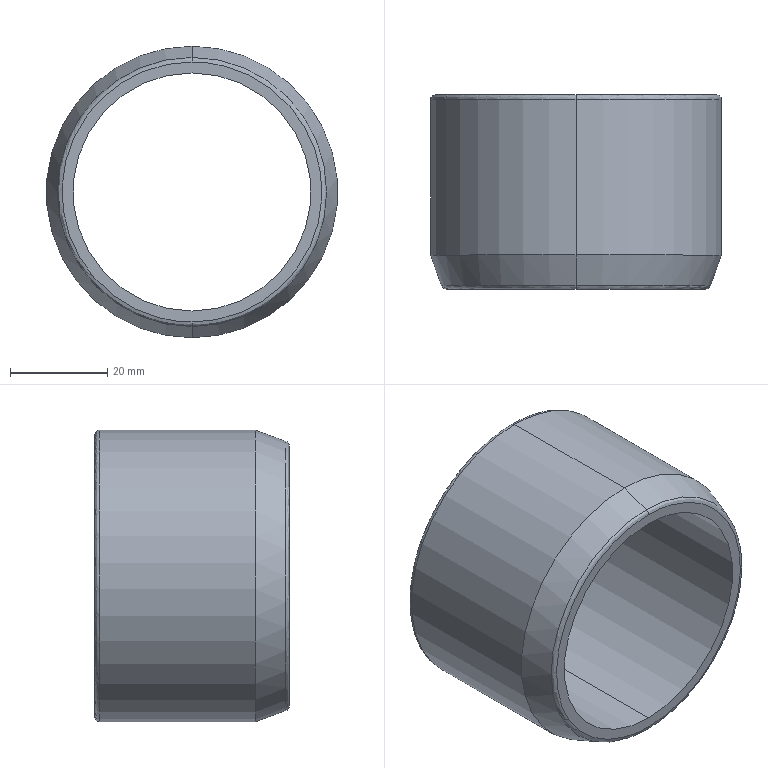Part | STEP file | 4. Piston Cap | 1 solid | 12 faces | box 60 x 40 x 60 mm | volume 35974 mm3 | spline 4 | cylinder 4 | cone 2 | plane 2 | commonest cylinder face diameters 49 x2 60 x2
STEP:
#1=CARTESIAN_POINT('',(0.,0.,26.752));
#2=VERTEX_POINT('',#1);
#3=CARTESIAN_POINT('',(0.,0.,-26.752));
#4=VERTEX_POINT('',#3);
#5=CARTESIAN_POINT('',(0.,0.,26.752));
#6=CARTESIAN_POINT('',(-0.818,0.,26.752));
#7=CARTESIAN_POINT('',(-2.04,0.,26.696));
#8=CARTESIAN_POINT('',(-3.457,0.,26.533));
#9=CARTESIAN_POINT('',(-4.163,0.,26.428));
#10=CARTESIAN_POINT('',(-4.516,0.,26.368));
#11=CARTESIAN_POINT('',(-4.692,0.,26.337));
#12=CARTESIAN_POINT('',(-4.767,0.,26.324));
#13=CARTESIAN_POINT('',(-4.818,0.,26.315));
#14=CARTESIAN_POINT('',(-4.841,0.,26.31));
#15=CARTESIAN_POINT('',(-5.721,0.,26.148));
#16=CARTESIAN_POINT('',(-6.983,0.,25.85));
#17=CARTESIAN_POINT('',(-8.425,0.,25.397));
#18=CARTESIAN_POINT('',(-9.139,0.,25.144));
#19=CARTESIAN_POINT('',(-9.494,0.,25.011));
#20=CARTESIAN_POINT('',(-9.671,0.,24.943));
#21=CARTESIAN_POINT('',(-9.746,0.,24.913));
#22=CARTESIAN_POINT('',(-9.797,0.,24.894));
#23=CARTESIAN_POINT('',(-9.821,0.,24.884));
#24=CARTESIAN_POINT('',(-10.688,0.,24.541));
#25=CARTESIAN_POINT('',(-11.917,0.,23.981));
#26=CARTESIAN_POINT('',(-13.296,0.,23.222));
#27=CARTESIAN_POINT('',(-13.972,0.,22.815));
#28=CARTESIAN_POINT('',(-14.307,0.,22.606));
#29=CARTESIAN_POINT('',(-14.449,0.,22.514));
#30=CARTESIAN_POINT('',(-14.544,0.,22.453));
#31=CARTESIAN_POINT('',(-14.591,0.,22.423));
#32=CARTESIAN_POINT('',(-16.184,0.,21.381));
#33=CARTESIAN_POINT('',(-17.611,0.,20.222));
#34=CARTESIAN_POINT('',(-19.569,0.,18.264));
#35=CARTESIAN_POINT('',(-20.493,0.,17.239));
#36=CARTESIAN_POINT('',(-21.475,0.,15.965));
#37=CARTESIAN_POINT('',(-21.941,0.,15.309));
#38=CARTESIAN_POINT('',(-22.168,0.,14.976));
#39=CARTESIAN_POINT('',(-22.264,0.,14.832));
#40=CARTESIAN_POINT('',(-22.328,0.,14.735));
#41=CARTESIAN_POINT('',(-22.36,0.,14.686));
#42=CARTESIAN_POINT('',(-22.886,0.,13.882));
#43=CARTESIAN_POINT('',(-23.567,0.,12.716));
#44=CARTESIAN_POINT('',(-24.256,0.,11.3));
#45=CARTESIAN_POINT('',(-24.574,0.,10.578));
#46=CARTESIAN_POINT('',(-24.726,0.,10.214));
#47=CARTESIAN_POINT('',(-24.8,0.,10.031));
#48=CARTESIAN_POINT('',(-24.832,0.,9.952));
#49=CARTESIAN_POINT('',(-24.853,0.,9.9));
#50=CARTESIAN_POINT('',(-24.864,0.,9.872));
#51=CARTESIAN_POINT('',(-25.193,0.,9.041));
#52=CARTESIAN_POINT('',(-25.611,0.,7.813));
#53=CARTESIAN_POINT('',(-25.994,0.,6.351));
#54=CARTESIAN_POINT('',(-26.158,0.,5.612));
#55=CARTESIAN_POINT('',(-26.234,0.,5.241));
#56=CARTESIAN_POINT('',(-26.27,0.,5.054));
#57=CARTESIAN_POINT('',(-26.285,0.,4.974));
#58=CARTESIAN_POINT('',(-26.295,0.,4.921));
#59=CARTESIAN_POINT('',(-26.301,0.,4.893));
#60=CARTESIAN_POINT('',(-26.603,0.,3.259));
#61=CARTESIAN_POINT('',(-26.752,0.,1.636));
#62=CARTESIAN_POINT('',(-26.752,0.,-0.818));
#63=CARTESIAN_POINT('',(-26.696,0.,-2.04));
#64=CARTESIAN_POINT('',(-26.533,0.,-3.457));
#65=CARTESIAN_POINT('',(-26.428,0.,-4.163));
#66=CARTESIAN_POINT('',(-26.368,0.,-4.516));
#67=CARTESIAN_POINT('',(-26.337,0.,-4.692));
#68=CARTESIAN_POINT('',(-26.324,0.,-4.767));
#69=CARTESIAN_POINT('',(-26.315,0.,-4.818));
#70=CARTESIAN_POINT('',(-26.31,0.,-4.841));
#71=CARTESIAN_POINT('',(-26.148,0.,-5.721));
#72=CARTESIAN_POINT('',(-25.85,0.,-6.983));
#73=CARTESIAN_POINT('',(-25.397,0.,-8.425));
#74=CARTESIAN_POINT('',(-25.144,0.,-9.139));
#75=CARTESIAN_POINT('',(-25.011,0.,-9.494));
#76=CARTESIAN_POINT('',(-24.943,0.,-9.671));
#77=CARTESIAN_POINT('',(-24.913,0.,-9.746));
#78=CARTESIAN_POINT('',(-24.894,0.,-9.797));
#79=CARTESIAN_POINT('',(-24.884,0.,-9.821));
#80=CARTESIAN_POINT('',(-24.541,0.,-10.688));
#81=CARTESIAN_POINT('',(-23.981,0.,-11.917));
#82=CARTESIAN_POINT('',(-23.222,0.,-13.296));
#83=CARTESIAN_POINT('',(-22.815,0.,-13.972));
#84=CARTESIAN_POINT('',(-22.606,0.,-14.307));
#85=CARTESIAN_POINT('',(-22.514,0.,-14.449));
#86=CARTESIAN_POINT('',(-22.453,0.,-14.544));
#87=CARTESIAN_POINT('',(-22.423,0.,-14.591));
#88=CARTESIAN_POINT('',(-21.381,0.,-16.184));
#89=CARTESIAN_POINT('',(-20.222,0.,-17.611));
#90=CARTESIAN_POINT('',(-18.264,0.,-19.569));
#91=CARTESIAN_POINT('',(-17.239,0.,-20.493));
#92=CARTESIAN_POINT('',(-15.965,0.,-21.475));
#93=CARTESIAN_POINT('',(-15.309,0.,-21.941));
#94=CARTESIAN_POINT('',(-14.976,0.,-22.168));
#95=CARTESIAN_POINT('',(-14.832,0.,-22.264));
#96=CARTESIAN_POINT('',(-14.735,0.,-22.328));
#97=CARTESIAN_POINT('',(-14.686,0.,-22.36));
#98=CARTESIAN_POINT('',(-13.882,0.,-22.886));
#99=CARTESIAN_POINT('',(-12.716,0.,-23.567));
#100=CARTESIAN_POINT('',(-11.3,0.,-24.256));
#101=CARTESIAN_POINT('',(-10.578,0.,-24.574));
#102=CARTESIAN_POINT('',(-10.214,0.,-24.726));
#103=CARTESIAN_POINT('',(-10.031,0.,-24.8));
#104=CARTESIAN_POINT('',(-9.952,0.,-24.832));
#105=CARTESIAN_POINT('',(-9.9,0.,-24.853));
#106=CARTESIAN_POINT('',(-9.872,0.,-24.864));
#107=CARTESIAN_POINT('',(-9.041,0.,-25.193));
#108=CARTESIAN_POINT('',(-7.813,0.,-25.611));
#109=CARTESIAN_POINT('',(-6.351,0.,-25.994));
#110=CARTESIAN_POINT('',(-5.612,0.,-26.158));
#111=CARTESIAN_POINT('',(-5.241,0.,-26.234));
#112=CARTESIAN_POINT('',(-5.054,0.,-26.27));
#113=CARTESIAN_POINT('',(-4.974,0.,-26.285));
#114=CARTESIAN_POINT('',(-4.921,0.,-26.295));
#115=CARTESIAN_POINT('',(-4.893,0.,-26.301));
#116=CARTESIAN_POINT('',(-3.259,0.,-26.603));
#117=CARTESIAN_POINT('',(-1.636,0.,-26.752));
#118=CARTESIAN_POINT('',(0.,0.,-26.752));
#119=B_SPLINE_CURVE_WITH_KNOTS('',3,(#5,#6,#7,#8,#9,#10,#11,#12,#13,#14,#15,#16,#17,#18,#19,#20,#21,#22,#23,#24,#25,#26,#27,#28,#29,#30,#31,#32,#33,#34,#35,#36,#37,#38,#39,#40,#41,#42,#43,#44,#45,#46,#47,#48,#49,#50,#51,#52,#53,#54,#55,#56,#57,#58,#59,#60,#61,#62,#63,#64,#65,#66,#67,#68,#69,#70,#71,#72,#73,#74,#75,#76,#77,#78,#79,#80,#81,#82,#83,#84,#85,#86,#87,#88,#89,#90,#91,#92,#93,#94,#95,#96,#97,#98,#99,#100,#101,#102,#103,#104,#105,#106,#107,#108,#109,#110,#111,#112,#113,#114,#115,#116,#117,#118),.UNSPECIFIED.,.F.,.F.,(4,1,1,1,1,1,2,2,1,1,1,1,1,2,2,1,1,1,1,2,2,2,1,1,1,1,2,2,1,1,1,1,1,2,2,1,1,1,1,1,2,2,2,1,1,1,1,1,2,2,1,1,1,1,1,2,2,1,1,1,1,2,2,2,1,1,1,1,2,2,1,1,1,1,1,2,2,1,1,1,1,1,2,2,4),(0.5,0.5156,0.5234,0.5273,0.5293,0.5303,0.5308,0.5312,0.5469,0.5547,0.5586,0.5605,0.5615,0.562,0.5625,0.5781,0.5859,0.5898,0.5918,0.5928,0.5938,0.625,0.6406,0.6484,0.6523,0.6543,0.6553,0.6563,0.6719,0.6797,0.6836,0.6855,0.6865,0.687,0.6875,0.7031,0.7109,0.7148,0.7168,0.7178,0.7183,0.7188,0.75,0.7656,0.7734,0.7773,0.7793,0.7803,0.7808,0.7813,0.7969,0.8047,0.8086,0.8105,0.8115,0.812,0.8125,0.8281,0.8359,0.8398,0.8418,0.8428,0.8438,0.875,0.8906,0.8984,0.9023,0.9043,0.9053,0.9063,0.9219,0.9297,0.9336,0.9355,0.9365,0.937,0.9375,0.9531,0.9609,0.9648,0.9668,0.9678,0.9683,0.9687,1.),.UNSPECIFIED.);
#120=EDGE_CURVE('',#2,#4,#119,.T.);
#121=ORIENTED_EDGE('',*,*,#120,.F.);
#122=CARTESIAN_POINT('',(0.,0.658,27.692));
#123=VERTEX_POINT('',#122);
#124=CARTESIAN_POINT('',(0.,1.,26.752));
#125=DIRECTION('',(-1.,0.,0.));
#126=DIRECTION('',(0.,0.,1.));
#127=AXIS2_PLACEMENT_3D('',#124,#125,#126);
#128=CIRCLE('',#127,1.);
#129=EDGE_CURVE('',#2,#123,#128,.T.);
#130=ORIENTED_EDGE('',*,*,#129,.T.);
#131=CARTESIAN_POINT('',(0.,0.658,-27.692));
#132=VERTEX_POINT('',#131);
#133=CARTESIAN_POINT('',(0.,0.658,0.));
#134=DIRECTION('',(0.,-1.,0.));
#135=DIRECTION('',(0.,0.,-1.));
#136=AXIS2_PLACEMENT_3D('',#133,#134,#135);
#137=CIRCLE('',#136,27.692);
#138=EDGE_CURVE('',#123,#132,#137,.T.);
#139=ORIENTED_EDGE('',*,*,#138,.T.);
#140=CARTESIAN_POINT('',(0.,1.,-26.752));
#141=DIRECTION('',(1.,0.,0.));
#142=DIRECTION('',(0.,0.,-1.));
#143=AXIS2_PLACEMENT_3D('',#140,#141,#142);
#144=CIRCLE('',#143,1.);
#145=EDGE_CURVE('',#4,#132,#144,.T.);
#146=ORIENTED_EDGE('',*,*,#145,.F.);
#147=EDGE_LOOP('',(#121,#130,#139,#146));
#148=FACE_OUTER_BOUND('',#147,.T.);
#149=CARTESIAN_POINT('',(0.,0.,26.752));
#150=CARTESIAN_POINT('',(-53.504,0.,26.752));
#151=CARTESIAN_POINT('',(-53.504,0.,-26.752));
#152=CARTESIAN_POINT('',(0.,0.,-26.752));
#153=CARTESIAN_POINT('',(0.,0.,27.187));
#154=CARTESIAN_POINT('',(-54.374,0.,27.187));
#155=CARTESIAN_POINT('',(-54.374,0.,-27.187));
#156=CARTESIAN_POINT('',(0.,0.,-27.187));
#157=CARTESIAN_POINT('',(0.,0.2494,27.543));
#158=CARTESIAN_POINT('',(-55.086,0.2494,27.543));
#159=CARTESIAN_POINT('',(-55.086,0.2494,-27.543));
#160=CARTESIAN_POINT('',(0.,0.2494,-27.543));
#161=CARTESIAN_POINT('',(0.,0.658,27.692));
#162=CARTESIAN_POINT('',(-55.383,0.658,27.692));
#163=CARTESIAN_POINT('',(-55.383,0.658,-27.692));
#164=CARTESIAN_POINT('',(0.,0.658,-27.692));
#165=(BOUNDED_SURFACE()B_SPLINE_SURFACE(3,3,((#149,#150,#151,#152),(#153,#154,#155,#156),(#157,#158,#159,#160),(#161,#162,#163,#164)),.UNSPECIFIED.,.F.,.F.,.F.)B_SPLINE_SURFACE_WITH_KNOTS((4,4),(4,4),(0.,1.),(0.,1.),.UNSPECIFIED.)GEOMETRIC_REPRESENTATION_ITEM()RATIONAL_B_SPLINE_SURFACE(((1.,0.3333,0.3333,1.),(0.8794,0.2931,0.2931,0.8794),(0.8794,0.2931,0.2931,0.8794),(1.,0.3333,0.3333,1.)))REPRESENTATION_ITEM('')SURFACE());
#166=ADVANCED_FACE('',(#148),#165,.T.);
#167=CARTESIAN_POINT('',(0.,39.,-30.));
#168=VERTEX_POINT('',#167);
#169=CARTESIAN_POINT('',(0.,39.,30.));
#170=VERTEX_POINT('',#169);
#171=CARTESIAN_POINT('',(0.,39.,0.));
#172=DIRECTION('',(0.,1.,0.));
#173=DIRECTION('',(0.,0.,-1.));
#174=AXIS2_PLACEMENT_3D('',#171,#172,#173);
#175=CIRCLE('',#174,30.);
#176=EDGE_CURVE('',#168,#170,#175,.T.);
#177=ORIENTED_EDGE('',*,*,#176,.T.);
#178=CARTESIAN_POINT('',(0.,40.,29.));
#179=VERTEX_POINT('',#178);
#180=CARTESIAN_POINT('',(0.,39.,29.));
#181=DIRECTION('',(-1.,0.,0.));
#182=DIRECTION('',(0.,0.,1.));
#183=AXIS2_PLACEMENT_3D('',#180,#181,#182);
#184=CIRCLE('',#183,1.);
#185=EDGE_CURVE('',#170,#179,#184,.T.);
#186=ORIENTED_EDGE('',*,*,#185,.T.);
#187=CARTESIAN_POINT('',(0.,40.,-29.));
#188=VERTEX_POINT('',#187);
#189=CARTESIAN_POINT('',(0.,40.,29.));
#190=CARTESIAN_POINT('',(-58.,40.,29.));
#191=CARTESIAN_POINT('',(-58.,40.,-29.));
#192=CARTESIAN_POINT('',(0.,40.,-29.));
#193=(BOUNDED_CURVE()B_SPLINE_CURVE(3,(#189,#190,#191,#192),.UNSPECIFIED.,.F.,.F.)B_SPLINE_CURVE_WITH_KNOTS((4,4),(0.5,1.),.UNSPECIFIED.)CURVE()GEOMETRIC_REPRESENTATION_ITEM()RATIONAL_B_SPLINE_CURVE((1.,0.3333,0.3333,1.))REPRESENTATION_ITEM(''));
#194=EDGE_CURVE('',#179,#188,#193,.T.);
#195=ORIENTED_EDGE('',*,*,#194,.T.);
#196=CARTESIAN_POINT('',(0.,39.,-29.));
#197=DIRECTION('',(1.,0.,0.));
#198=DIRECTION('',(0.,0.,-1.));
#199=AXIS2_PLACEMENT_3D('',#196,#197,#198);
#200=CIRCLE('',#199,1.);
#201=EDGE_CURVE('',#168,#188,#200,.T.);
#202=ORIENTED_EDGE('',*,*,#201,.F.);
#203=EDGE_LOOP('',(#177,#186,#195,#202));
#204=FACE_OUTER_BOUND('',#203,.T.);
#205=CARTESIAN_POINT('',(0.,39.,30.));
#206=CARTESIAN_POINT('',(-60.,39.,30.));
#207=CARTESIAN_POINT('',(-60.,39.,-30.));
#208=CARTESIAN_POINT('',(0.,39.,-30.));
#209=CARTESIAN_POINT('',(0.,39.586,30.));
#210=CARTESIAN_POINT('',(-60.,39.586,30.));
#211=CARTESIAN_POINT('',(-60.,39.586,-30.));
#212=CARTESIAN_POINT('',(0.,39.586,-30.));
#213=CARTESIAN_POINT('',(0.,40.,29.586));
#214=CARTESIAN_POINT('',(-59.172,40.,29.586));
#215=CARTESIAN_POINT('',(-59.172,40.,-29.586));
#216=CARTESIAN_POINT('',(0.,40.,-29.586));
#217=CARTESIAN_POINT('',(0.,40.,29.));
#218=CARTESIAN_POINT('',(-58.,40.,29.));
#219=CARTESIAN_POINT('',(-58.,40.,-29.));
#220=CARTESIAN_POINT('',(0.,40.,-29.));
#221=(BOUNDED_SURFACE()B_SPLINE_SURFACE(3,3,((#205,#206,#207,#208),(#209,#210,#211,#212),(#213,#214,#215,#216),(#217,#218,#219,#220)),.UNSPECIFIED.,.F.,.F.,.F.)B_SPLINE_SURFACE_WITH_KNOTS((4,4),(4,4),(0.,1.),(0.,1.),.UNSPECIFIED.)GEOMETRIC_REPRESENTATION_ITEM()RATIONAL_B_SPLINE_SURFACE(((1.,0.3333,0.3333,1.),(0.8047,0.2682,0.2682,0.8047),(0.8047,0.2682,0.2682,0.8047),(1.,0.3333,0.3333,1.)))REPRESENTATION_ITEM('')SURFACE());
#222=ADVANCED_FACE('',(#204),#221,.T.);
#223=CARTESIAN_POINT('',(0.,40.,24.5));
#224=VERTEX_POINT('',#223);
#225=CARTESIAN_POINT('',(0.,40.,-24.5));
#226=VERTEX_POINT('',#225);
#227=CARTESIAN_POINT('',(0.,40.,0.));
#228=DIRECTION('',(0.,-1.,0.));
#229=DIRECTION('',(0.,0.,-1.));
#230=AXIS2_PLACEMENT_3D('',#227,#228,#229);
#231=CIRCLE('',#230,24.5);
#232=EDGE_CURVE('',#224,#226,#231,.T.);
#233=ORIENTED_EDGE('',*,*,#232,.F.);
#234=CARTESIAN_POINT('',(0.,0.,24.5));
#235=VERTEX_POINT('',#234);
#236=CARTESIAN_POINT('',(0.,40.,24.5));
#237=DIRECTION('',(0.,-1.,0.));
#238=VECTOR('',#237,1000.);
#239=LINE('',#236,#238);
#240=EDGE_CURVE('',#224,#235,#239,.T.);
#241=ORIENTED_EDGE('',*,*,#240,.T.);
#242=CARTESIAN_POINT('',(0.,0.,-24.5));
#243=VERTEX_POINT('',#242);
#244=CARTESIAN_POINT('',(0.,0.,0.));
#245=DIRECTION('',(0.,1.,0.));
#246=DIRECTION('',(0.,0.,-1.));
#247=AXIS2_PLACEMENT_3D('',#244,#245,#246);
#248=CIRCLE('',#247,24.5);
#249=EDGE_CURVE('',#243,#235,#248,.T.);
#250=ORIENTED_EDGE('',*,*,#249,.F.);
#251=CARTESIAN_POINT('',(0.,40.,-24.5));
#252=DIRECTION('',(0.,-1.,0.));
#253=VECTOR('',#252,1000.);
#254=LINE('',#251,#253);
#255=EDGE_CURVE('',#226,#243,#254,.T.);
#256=ORIENTED_EDGE('',*,*,#255,.F.);
#257=EDGE_LOOP('',(#233,#241,#250,#256));
#258=FACE_OUTER_BOUND('',#257,.T.);
#259=CARTESIAN_POINT('',(0.,40.,0.));
#260=DIRECTION('',(0.,-1.,0.));
#261=DIRECTION('',(0.,0.,-1.));
#262=AXIS2_PLACEMENT_3D('',#259,#260,#261);
#263=CYLINDRICAL_SURFACE('',#262,24.5);
#264=ADVANCED_FACE('',(#258),#263,.F.);
#265=CARTESIAN_POINT('',(0.,0.658,0.));
#266=DIRECTION('',(0.,-1.,0.));
#267=DIRECTION('',(0.,0.,-1.));
#268=AXIS2_PLACEMENT_3D('',#265,#266,#267);
#269=CIRCLE('',#268,27.692);
#270=EDGE_CURVE('',#132,#123,#269,.T.);
#271=ORIENTED_EDGE('',*,*,#270,.F.);
#272=CARTESIAN_POINT('',(0.,7.,-30.));
#273=VERTEX_POINT('',#272);
#274=CARTESIAN_POINT('',(0.,7.,-30.));
#275=DIRECTION('',(0.,0.9397,-0.342));
#276=VECTOR('',#275,1000.);
#277=LINE('',#274,#276);
#278=EDGE_CURVE('',#132,#273,#277,.T.);
#279=ORIENTED_EDGE('',*,*,#278,.T.);
#280=CARTESIAN_POINT('',(0.,7.,30.));
#281=VERTEX_POINT('',#280);
#282=CARTESIAN_POINT('',(0.,7.,0.));
#283=DIRECTION('',(0.,-1.,0.));
#284=DIRECTION('',(0.,0.,1.));
#285=AXIS2_PLACEMENT_3D('',#282,#283,#284);
#286=CIRCLE('',#285,30.);
#287=EDGE_CURVE('',#273,#281,#286,.T.);
#288=ORIENTED_EDGE('',*,*,#287,.T.);
#289=CARTESIAN_POINT('',(0.,7.,30.));
#290=DIRECTION('',(0.,0.9397,0.342));
#291=VECTOR('',#290,1000.);
#292=LINE('',#289,#291);
#293=EDGE_CURVE('',#123,#281,#292,.T.);
#294=ORIENTED_EDGE('',*,*,#293,.F.);
#295=EDGE_LOOP('',(#271,#279,#288,#294));
#296=FACE_OUTER_BOUND('',#295,.T.);
#297=CARTESIAN_POINT('',(0.,7.,0.));
#298=DIRECTION('',(0.,1.,0.));
#299=DIRECTION('',(0.,0.,1.));
#300=AXIS2_PLACEMENT_3D('',#297,#298,#299);
#301=CONICAL_SURFACE('',#300,30.,0.3491);
#302=ADVANCED_FACE('',(#296),#301,.T.);
#303=CARTESIAN_POINT('',(0.,39.,0.));
#304=DIRECTION('',(0.,1.,0.));
#305=DIRECTION('',(0.,0.,-1.));
#306=AXIS2_PLACEMENT_3D('',#303,#304,#305);
#307=CIRCLE('',#306,30.);
#308=EDGE_CURVE('',#170,#168,#307,.T.);
#309=ORIENTED_EDGE('',*,*,#308,.F.);
#310=CARTESIAN_POINT('',(0.,40.,30.));
#311=DIRECTION('',(0.,-1.,0.));
#312=VECTOR('',#311,1000.);
#313=LINE('',#310,#312);
#314=EDGE_CURVE('',#170,#281,#313,.T.);
#315=ORIENTED_EDGE('',*,*,#314,.T.);
#316=ORIENTED_EDGE('',*,*,#287,.F.);
#317=CARTESIAN_POINT('',(0.,40.,-30.));
#318=DIRECTION('',(0.,-1.,0.));
#319=VECTOR('',#318,1000.);
#320=LINE('',#317,#319);
#321=EDGE_CURVE('',#168,#273,#320,.T.);
#322=ORIENTED_EDGE('',*,*,#321,.F.);
#323=EDGE_LOOP('',(#309,#315,#316,#322));
#324=FACE_OUTER_BOUND('',#323,.T.);
#325=CARTESIAN_POINT('',(0.,40.,0.));
#326=DIRECTION('',(0.,-1.,0.));
#327=DIRECTION('',(0.,0.,-1.));
#328=AXIS2_PLACEMENT_3D('',#325,#326,#327);
#329=CYLINDRICAL_SURFACE('',#328,30.);
#330=ADVANCED_FACE('',(#324),#329,.T.);
#331=ORIENTED_EDGE('',*,*,#240,.F.);
#332=CARTESIAN_POINT('',(0.,40.,0.));
#333=DIRECTION('',(0.,-1.,0.));
#334=DIRECTION('',(0.,0.,-1.));
#335=AXIS2_PLACEMENT_3D('',#332,#333,#334);
#336=CIRCLE('',#335,24.5);
#337=EDGE_CURVE('',#226,#224,#336,.T.);
#338=ORIENTED_EDGE('',*,*,#337,.F.);
#339=ORIENTED_EDGE('',*,*,#255,.T.);
#340=CARTESIAN_POINT('',(0.,0.,0.));
#341=DIRECTION('',(0.,1.,0.));
#342=DIRECTION('',(0.,0.,-1.));
#343=AXIS2_PLACEMENT_3D('',#340,#341,#342);
#344=CIRCLE('',#343,24.5);
#345=EDGE_CURVE('',#235,#243,#344,.T.);
#346=ORIENTED_EDGE('',*,*,#345,.F.);
#347=EDGE_LOOP('',(#331,#338,#339,#346));
#348=FACE_OUTER_BOUND('',#347,.T.);
#349=CARTESIAN_POINT('',(0.,40.,0.));
#350=DIRECTION('',(0.,-1.,0.));
#351=DIRECTION('',(0.,0.,-1.));
#352=AXIS2_PLACEMENT_3D('',#349,#350,#351);
#353=CYLINDRICAL_SURFACE('',#352,24.5);
#354=ADVANCED_FACE('',(#348),#353,.F.);
#355=ORIENTED_EDGE('',*,*,#249,.T.);
#356=ORIENTED_EDGE('',*,*,#345,.T.);
#357=EDGE_LOOP('',(#355,#356));
#358=FACE_BOUND('',#357,.T.);
#359=CARTESIAN_POINT('',(0.,0.,-26.752));
#360=CARTESIAN_POINT('',(0.8181,0.,-26.752));
#361=CARTESIAN_POINT('',(2.04,0.,-26.696));
#362=CARTESIAN_POINT('',(3.457,0.,-26.533));
#363=CARTESIAN_POINT('',(4.163,0.,-26.428));
#364=CARTESIAN_POINT('',(4.516,0.,-26.368));
#365=CARTESIAN_POINT('',(4.692,0.,-26.337));
#366=CARTESIAN_POINT('',(4.767,0.,-26.324));
#367=CARTESIAN_POINT('',(4.818,0.,-26.315));
#368=CARTESIAN_POINT('',(4.841,0.,-26.31));
#369=CARTESIAN_POINT('',(5.721,0.,-26.148));
#370=CARTESIAN_POINT('',(6.983,0.,-25.85));
#371=CARTESIAN_POINT('',(8.425,0.,-25.397));
#372=CARTESIAN_POINT('',(9.139,0.,-25.144));
#373=CARTESIAN_POINT('',(9.494,0.,-25.011));
#374=CARTESIAN_POINT('',(9.671,0.,-24.943));
#375=CARTESIAN_POINT('',(9.746,0.,-24.913));
#376=CARTESIAN_POINT('',(9.797,0.,-24.894));
#377=CARTESIAN_POINT('',(9.821,0.,-24.884));
#378=CARTESIAN_POINT('',(10.688,0.,-24.541));
#379=CARTESIAN_POINT('',(11.917,0.,-23.981));
#380=CARTESIAN_POINT('',(13.296,0.,-23.222));
#381=CARTESIAN_POINT('',(13.972,0.,-22.815));
#382=CARTESIAN_POINT('',(14.307,0.,-22.606));
#383=CARTESIAN_POINT('',(14.449,0.,-22.514));
#384=CARTESIAN_POINT('',(14.544,0.,-22.453));
#385=CARTESIAN_POINT('',(14.591,0.,-22.423));
#386=CARTESIAN_POINT('',(16.184,0.,-21.381));
#387=CARTESIAN_POINT('',(17.611,0.,-20.222));
#388=CARTESIAN_POINT('',(19.569,0.,-18.264));
#389=CARTESIAN_POINT('',(20.493,0.,-17.239));
#390=CARTESIAN_POINT('',(21.475,0.,-15.965));
#391=CARTESIAN_POINT('',(21.941,0.,-15.309));
#392=CARTESIAN_POINT('',(22.168,0.,-14.976));
#393=CARTESIAN_POINT('',(22.264,0.,-14.832));
#394=CARTESIAN_POINT('',(22.328,0.,-14.735));
#395=CARTESIAN_POINT('',(22.36,0.,-14.686));
#396=CARTESIAN_POINT('',(22.886,0.,-13.882));
#397=CARTESIAN_POINT('',(23.567,0.,-12.716));
#398=CARTESIAN_POINT('',(24.256,0.,-11.3));
#399=CARTESIAN_POINT('',(24.574,0.,-10.578));
#400=CARTESIAN_POINT('',(24.726,0.,-10.214));
#401=CARTESIAN_POINT('',(24.8,0.,-10.031));
#402=CARTESIAN_POINT('',(24.832,0.,-9.952));
#403=CARTESIAN_POINT('',(24.853,0.,-9.9));
#404=CARTESIAN_POINT('',(24.864,0.,-9.872));
#405=CARTESIAN_POINT('',(25.193,0.,-9.041));
#406=CARTESIAN_POINT('',(25.611,0.,-7.813));
#407=CARTESIAN_POINT('',(25.994,0.,-6.351));
#408=CARTESIAN_POINT('',(26.158,0.,-5.612));
#409=CARTESIAN_POINT('',(26.234,0.,-5.241));
#410=CARTESIAN_POINT('',(26.27,0.,-5.054));
#411=CARTESIAN_POINT('',(26.285,0.,-4.974));
#412=CARTESIAN_POINT('',(26.295,0.,-4.921));
#413=CARTESIAN_POINT('',(26.301,0.,-4.893));
#414=CARTESIAN_POINT('',(26.603,0.,-3.259));
#415=CARTESIAN_POINT('',(26.752,0.,-1.636));
#416=CARTESIAN_POINT('',(26.752,0.,0.818));
#417=CARTESIAN_POINT('',(26.696,0.,2.04));
#418=CARTESIAN_POINT('',(26.533,0.,3.457));
#419=CARTESIAN_POINT('',(26.428,0.,4.163));
#420=CARTESIAN_POINT('',(26.368,0.,4.516));
#421=CARTESIAN_POINT('',(26.337,0.,4.692));
#422=CARTESIAN_POINT('',(26.324,0.,4.767));
#423=CARTESIAN_POINT('',(26.315,0.,4.818));
#424=CARTESIAN_POINT('',(26.31,0.,4.841));
#425=CARTESIAN_POINT('',(26.148,0.,5.721));
#426=CARTESIAN_POINT('',(25.85,0.,6.983));
#427=CARTESIAN_POINT('',(25.397,0.,8.425));
#428=CARTESIAN_POINT('',(25.144,0.,9.139));
#429=CARTESIAN_POINT('',(25.011,0.,9.494));
#430=CARTESIAN_POINT('',(24.943,0.,9.671));
#431=CARTESIAN_POINT('',(24.913,0.,9.746));
#432=CARTESIAN_POINT('',(24.894,0.,9.797));
#433=CARTESIAN_POINT('',(24.884,0.,9.821));
#434=CARTESIAN_POINT('',(24.541,0.,10.688));
#435=CARTESIAN_POINT('',(23.981,0.,11.917));
#436=CARTESIAN_POINT('',(23.222,0.,13.296));
#437=CARTESIAN_POINT('',(22.815,0.,13.972));
#438=CARTESIAN_POINT('',(22.606,0.,14.307));
#439=CARTESIAN_POINT('',(22.514,0.,14.449));
#440=CARTESIAN_POINT('',(22.453,0.,14.544));
#441=CARTESIAN_POINT('',(22.423,0.,14.591));
#442=CARTESIAN_POINT('',(21.381,0.,16.184));
#443=CARTESIAN_POINT('',(20.222,0.,17.611));
#444=CARTESIAN_POINT('',(18.264,0.,19.569));
#445=CARTESIAN_POINT('',(17.239,0.,20.493));
#446=CARTESIAN_POINT('',(15.965,0.,21.475));
#447=CARTESIAN_POINT('',(15.309,0.,21.941));
#448=CARTESIAN_POINT('',(14.976,0.,22.168));
#449=CARTESIAN_POINT('',(14.832,0.,22.264));
#450=CARTESIAN_POINT('',(14.735,0.,22.328));
#451=CARTESIAN_POINT('',(14.686,0.,22.36));
#452=CARTESIAN_POINT('',(13.882,0.,22.886));
#453=CARTESIAN_POINT('',(12.716,0.,23.567));
#454=CARTESIAN_POINT('',(11.3,0.,24.256));
#455=CARTESIAN_POINT('',(10.578,0.,24.574));
#456=CARTESIAN_POINT('',(10.214,0.,24.726));
#457=CARTESIAN_POINT('',(10.031,0.,24.8));
#458=CARTESIAN_POINT('',(9.952,0.,24.832));
#459=CARTESIAN_POINT('',(9.9,0.,24.853));
#460=CARTESIAN_POINT('',(9.872,0.,24.864));
#461=CARTESIAN_POINT('',(9.041,0.,25.193));
#462=CARTESIAN_POINT('',(7.813,0.,25.611));
#463=CARTESIAN_POINT('',(6.351,0.,25.994));
#464=CARTESIAN_POINT('',(5.612,0.,26.158));
#465=CARTESIAN_POINT('',(5.241,0.,26.234));
#466=CARTESIAN_POINT('',(5.054,0.,26.27));
#467=CARTESIAN_POINT('',(4.974,0.,26.285));
#468=CARTESIAN_POINT('',(4.921,0.,26.295));
#469=CARTESIAN_POINT('',(4.893,0.,26.301));
#470=CARTESIAN_POINT('',(3.259,0.,26.603));
#471=CARTESIAN_POINT('',(1.636,0.,26.752));
#472=CARTESIAN_POINT('',(0.,0.,26.752));
#473=B_SPLINE_CURVE_WITH_KNOTS('',3,(#359,#360,#361,#362,#363,#364,#365,#366,#367,#368,#369,#370,#371,#372,#373,#374,#375,#376,#377,#378,#379,#380,#381,#382,#383,#384,#385,#386,#387,#388,#389,#390,#391,#392,#393,#394,#395,#396,#397,#398,#399,#400,#401,#402,#403,#404,#405,#406,#407,#408,#409,#410,#411,#412,#413,#414,#415,#416,#417,#418,#419,#420,#421,#422,#423,#424,#425,#426,#427,#428,#429,#430,#431,#432,#433,#434,#435,#436,#437,#438,#439,#440,#441,#442,#443,#444,#445,#446,#447,#448,#449,#450,#451,#452,#453,#454,#455,#456,#457,#458,#459,#460,#461,#462,#463,#464,#465,#466,#467,#468,#469,#470,#471,#472),.UNSPECIFIED.,.F.,.F.,(4,1,1,1,1,1,2,2,1,1,1,1,1,2,2,1,1,1,1,2,2,2,1,1,1,1,2,2,1,1,1,1,1,2,2,1,1,1,1,1,2,2,2,1,1,1,1,1,2,2,1,1,1,1,1,2,2,1,1,1,1,2,2,2,1,1,1,1,2,2,1,1,1,1,1,2,2,1,1,1,1,1,2,2,4),(0.,0.01562,0.02344,0.02734,0.0293,0.03027,0.03076,0.03125,0.04687,0.05469,0.05859,0.06055,0.06152,0.06201,0.0625,0.07812,0.08594,0.08984,0.0918,0.09277,0.09375,0.125,0.1406,0.1484,0.1523,0.1543,0.1553,0.1562,0.1719,0.1797,0.1836,0.1855,0.1865,0.187,0.1875,0.2031,0.2109,0.2148,0.2168,0.2178,0.2183,0.2187,0.25,0.2656,0.2734,0.2773,0.2793,0.2803,0.2808,0.2812,0.2969,0.3047,0.3086,0.3105,0.3115,0.312,0.3125,0.3281,0.3359,0.3398,0.3418,0.3428,0.3437,0.375,0.3906,0.3984,0.4023,0.4043,0.4053,0.4062,0.4219,0.4297,0.4336,0.4355,0.4365,0.437,0.4375,0.4531,0.4609,0.4648,0.4668,0.4678,0.4683,0.4687,0.5),.UNSPECIFIED.);
#474=EDGE_CURVE('',#4,#2,#473,.T.);
#475=ORIENTED_EDGE('',*,*,#474,.T.);
#476=ORIENTED_EDGE('',*,*,#120,.T.);
#477=EDGE_LOOP('',(#475,#476));
#478=FACE_OUTER_BOUND('',#477,.T.);
#479=CARTESIAN_POINT('',(0.,0.,0.));
#480=DIRECTION('',(0.,-1.,0.));
#481=DIRECTION('',(0.,0.,-1.));
#482=AXIS2_PLACEMENT_3D('',#479,#480,#481);
#483=PLANE('',#482);
#484=ADVANCED_FACE('',(#358,#478),#483,.T.);
#485=ORIENTED_EDGE('',*,*,#337,.T.);
#486=ORIENTED_EDGE('',*,*,#232,.T.);
#487=EDGE_LOOP('',(#485,#486));
#488=FACE_BOUND('',#487,.T.);
#489=CARTESIAN_POINT('',(0.,40.,-29.));
#490=CARTESIAN_POINT('',(58.,40.,-29.));
#491=CARTESIAN_POINT('',(58.,40.,29.));
#492=CARTESIAN_POINT('',(0.,40.,29.));
#493=(BOUNDED_CURVE()B_SPLINE_CURVE(3,(#489,#490,#491,#492),.UNSPECIFIED.,.F.,.F.)B_SPLINE_CURVE_WITH_KNOTS((4,4),(0.,0.5),.UNSPECIFIED.)CURVE()GEOMETRIC_REPRESENTATION_ITEM()RATIONAL_B_SPLINE_CURVE((1.,0.3333,0.3333,1.))REPRESENTATION_ITEM(''));
#494=EDGE_CURVE('',#188,#179,#493,.T.);
#495=ORIENTED_EDGE('',*,*,#494,.F.);
#496=ORIENTED_EDGE('',*,*,#194,.F.);
#497=EDGE_LOOP('',(#495,#496));
#498=FACE_OUTER_BOUND('',#497,.T.);
#499=CARTESIAN_POINT('',(0.,40.,0.));
#500=DIRECTION('',(0.,-1.,0.));
#501=DIRECTION('',(0.,0.,-1.));
#502=AXIS2_PLACEMENT_3D('',#499,#500,#501);
#503=PLANE('',#502);
#504=ADVANCED_FACE('',(#488,#498),#503,.F.);
#505=ORIENTED_EDGE('',*,*,#129,.F.);
#506=ORIENTED_EDGE('',*,*,#474,.F.);
#507=ORIENTED_EDGE('',*,*,#145,.T.);
#508=ORIENTED_EDGE('',*,*,#270,.T.);
#509=EDGE_LOOP('',(#505,#506,#507,#508));
#510=FACE_OUTER_BOUND('',#509,.T.);
#511=CARTESIAN_POINT('',(0.,0.,-26.752));
#512=CARTESIAN_POINT('',(53.504,0.,-26.752));
#513=CARTESIAN_POINT('',(53.504,0.,26.752));
#514=CARTESIAN_POINT('',(0.,0.,26.752));
#515=CARTESIAN_POINT('',(0.,0.,-27.187));
#516=CARTESIAN_POINT('',(54.374,0.,-27.187));
#517=CARTESIAN_POINT('',(54.374,0.,27.187));
#518=CARTESIAN_POINT('',(0.,0.,27.187));
#519=CARTESIAN_POINT('',(0.,0.2494,-27.543));
#520=CARTESIAN_POINT('',(55.086,0.2494,-27.543));
#521=CARTESIAN_POINT('',(55.086,0.2494,27.543));
#522=CARTESIAN_POINT('',(0.,0.2494,27.543));
#523=CARTESIAN_POINT('',(0.,0.658,-27.692));
#524=CARTESIAN_POINT('',(55.383,0.658,-27.692));
#525=CARTESIAN_POINT('',(55.383,0.658,27.692));
#526=CARTESIAN_POINT('',(0.,0.658,27.692));
#527=(BOUNDED_SURFACE()B_SPLINE_SURFACE(3,3,((#511,#512,#513,#514),(#515,#516,#517,#518),(#519,#520,#521,#522),(#523,#524,#525,#526)),.UNSPECIFIED.,.F.,.F.,.F.)B_SPLINE_SURFACE_WITH_KNOTS((4,4),(4,4),(0.,1.),(0.,1.),.UNSPECIFIED.)GEOMETRIC_REPRESENTATION_ITEM()RATIONAL_B_SPLINE_SURFACE(((1.,0.3333,0.3333,1.),(0.8794,0.2931,0.2931,0.8794),(0.8794,0.2931,0.2931,0.8794),(1.,0.3333,0.3333,1.)))REPRESENTATION_ITEM('')SURFACE());
#528=ADVANCED_FACE('',(#510),#527,.T.);
#529=ORIENTED_EDGE('',*,*,#185,.F.);
#530=ORIENTED_EDGE('',*,*,#308,.T.);
#531=ORIENTED_EDGE('',*,*,#201,.T.);
#532=ORIENTED_EDGE('',*,*,#494,.T.);
#533=EDGE_LOOP('',(#529,#530,#531,#532));
#534=FACE_OUTER_BOUND('',#533,.T.);
#535=CARTESIAN_POINT('',(0.,39.,-30.));
#536=CARTESIAN_POINT('',(60.,39.,-30.));
#537=CARTESIAN_POINT('',(60.,39.,30.));
#538=CARTESIAN_POINT('',(0.,39.,30.));
#539=CARTESIAN_POINT('',(0.,39.586,-30.));
#540=CARTESIAN_POINT('',(60.,39.586,-30.));
#541=CARTESIAN_POINT('',(60.,39.586,30.));
#542=CARTESIAN_POINT('',(0.,39.586,30.));
#543=CARTESIAN_POINT('',(0.,40.,-29.586));
#544=CARTESIAN_POINT('',(59.172,40.,-29.586));
#545=CARTESIAN_POINT('',(59.172,40.,29.586));
#546=CARTESIAN_POINT('',(0.,40.,29.586));
#547=CARTESIAN_POINT('',(0.,40.,-29.));
#548=CARTESIAN_POINT('',(58.,40.,-29.));
#549=CARTESIAN_POINT('',(58.,40.,29.));
#550=CARTESIAN_POINT('',(0.,40.,29.));
#551=(BOUNDED_SURFACE()B_SPLINE_SURFACE(3,3,((#535,#536,#537,#538),(#539,#540,#541,#542),(#543,#544,#545,#546),(#547,#548,#549,#550)),.UNSPECIFIED.,.F.,.F.,.F.)B_SPLINE_SURFACE_WITH_KNOTS((4,4),(4,4),(0.,1.),(0.,1.),.UNSPECIFIED.)GEOMETRIC_REPRESENTATION_ITEM()RATIONAL_B_SPLINE_SURFACE(((1.,0.3333,0.3333,1.),(0.8047,0.2682,0.2682,0.8047),(0.8047,0.2682,0.2682,0.8047),(1.,0.3333,0.3333,1.)))REPRESENTATION_ITEM('')SURFACE());
#552=ADVANCED_FACE('',(#534),#551,.T.);
#553=ORIENTED_EDGE('',*,*,#278,.F.);
#554=ORIENTED_EDGE('',*,*,#138,.F.);
#555=ORIENTED_EDGE('',*,*,#293,.T.);
#556=CARTESIAN_POINT('',(0.,7.,0.));
#557=DIRECTION('',(0.,-1.,0.));
#558=DIRECTION('',(0.,0.,1.));
#559=AXIS2_PLACEMENT_3D('',#556,#557,#558);
#560=CIRCLE('',#559,30.);
#561=EDGE_CURVE('',#281,#273,#560,.T.);
#562=ORIENTED_EDGE('',*,*,#561,.T.);
#563=EDGE_LOOP('',(#553,#554,#555,#562));
#564=FACE_OUTER_BOUND('',#563,.T.);
#565=CARTESIAN_POINT('',(0.,7.,0.));
#566=DIRECTION('',(0.,1.,0.));
#567=DIRECTION('',(0.,0.,1.));
#568=AXIS2_PLACEMENT_3D('',#565,#566,#567);
#569=CONICAL_SURFACE('',#568,30.,0.3491);
#570=ADVANCED_FACE('',(#564),#569,.T.);
#571=ORIENTED_EDGE('',*,*,#314,.F.);
#572=ORIENTED_EDGE('',*,*,#176,.F.);
#573=ORIENTED_EDGE('',*,*,#321,.T.);
#574=ORIENTED_EDGE('',*,*,#561,.F.);
#575=EDGE_LOOP('',(#571,#572,#573,#574));
#576=FACE_OUTER_BOUND('',#575,.T.);
#577=CARTESIAN_POINT('',(0.,40.,0.));
#578=DIRECTION('',(0.,-1.,0.));
#579=DIRECTION('',(0.,0.,-1.));
#580=AXIS2_PLACEMENT_3D('',#577,#578,#579);
#581=CYLINDRICAL_SURFACE('',#580,30.);
#582=ADVANCED_FACE('',(#576),#581,.T.);
#583=CLOSED_SHELL('',(#166,#222,#264,#302,#330,#354,#484,#504,#528,#552,#570,#582));
#584=MANIFOLD_SOLID_BREP('',#583);
#585=CARTESIAN_POINT('',(0.,0.,0.));
#586=DIRECTION('',(0.,0.,1.));
#587=DIRECTION('',(1.,0.,0.));
#588=AXIS2_PLACEMENT_3D('',#585,#586,#587);
#589=(LENGTH_UNIT()NAMED_UNIT(*)SI_UNIT(.MILLI.,.METRE.));
#590=UNCERTAINTY_MEASURE_WITH_UNIT(LENGTH_MEASURE(0.00001),#589,'','');
#591=(NAMED_UNIT(*)PLANE_ANGLE_UNIT()SI_UNIT($,.RADIAN.));
#592=(NAMED_UNIT(*)SI_UNIT($,.STERADIAN.)SOLID_ANGLE_UNIT());
#593=(GEOMETRIC_REPRESENTATION_CONTEXT(3)GLOBAL_UNCERTAINTY_ASSIGNED_CONTEXT((#590))GLOBAL_UNIT_ASSIGNED_CONTEXT((#589,#591,#592))REPRESENTATION_CONTEXT('',''));
#594=ADVANCED_BREP_SHAPE_REPRESENTATION('',(#584,#588),#593);